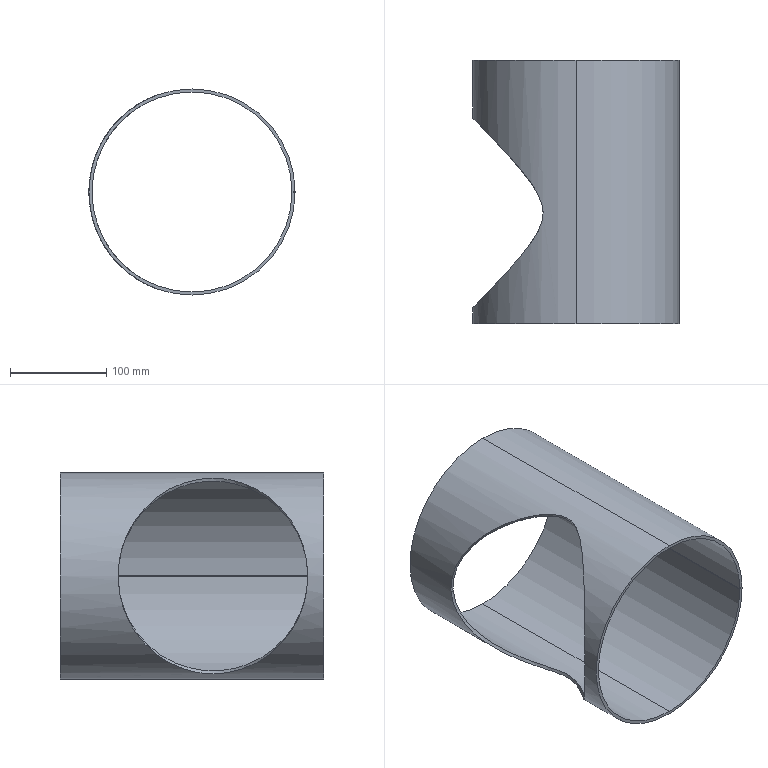Part | SolidWorks | features BaseBody 1 | 1 solid | 20 faces | box 213.699 x 273 x 213.7 mm | volume 459194 mm3 | spline 8 | cylinder 6 | plane 6 | commonest cylinder face diameters 207.3 x3 213.7 x3